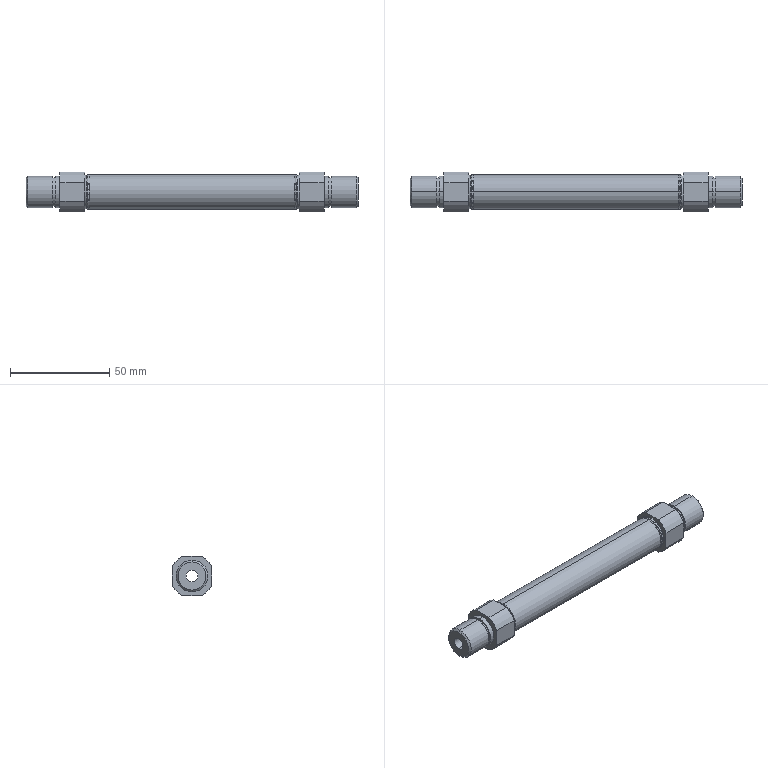Part | SolidWorks | features BaseBody 1 | 1 solid | 84 faces | box 167 x 20 x 20 mm | volume 22187 mm3 | cylinder 36 | plane 24 | cone 16 | spline 8 | commonest cylinder face diameters 16 x8 22 x8 17.4 x6 4.134 x4 6 x4 14.4 x4